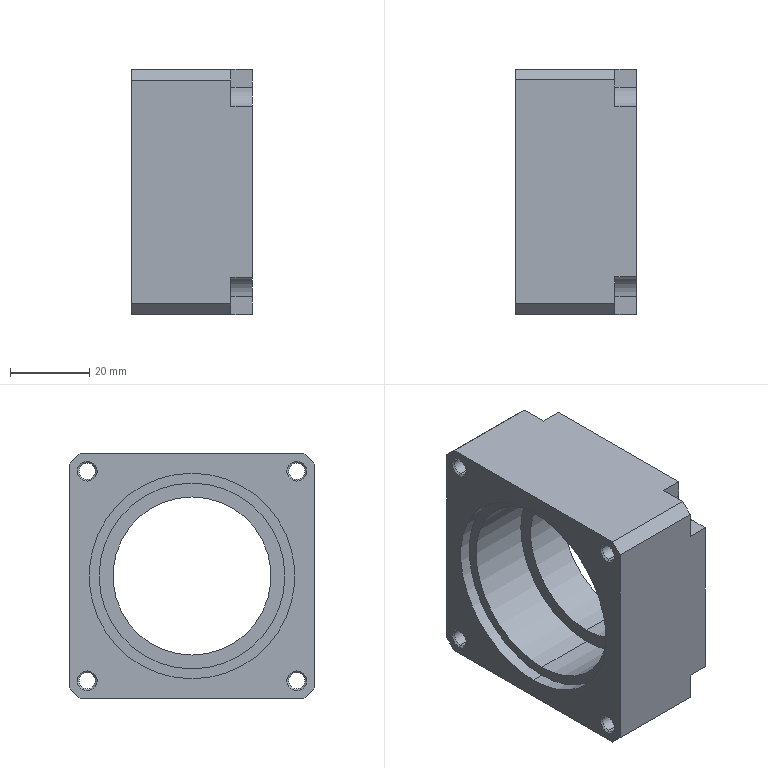Part | STEP file | _MoAd-PLE60x-PAS42 B-2 | 1 solid | 73 faces | box 30.5 x 62 x 62 mm | volume 64839 mm3 | plane 29 | cylinder 28 | cone 16 | commonest cylinder face diameters 4.134 x8 5.5 x8 10 x4 8.5 x2 40 x2 47 x2